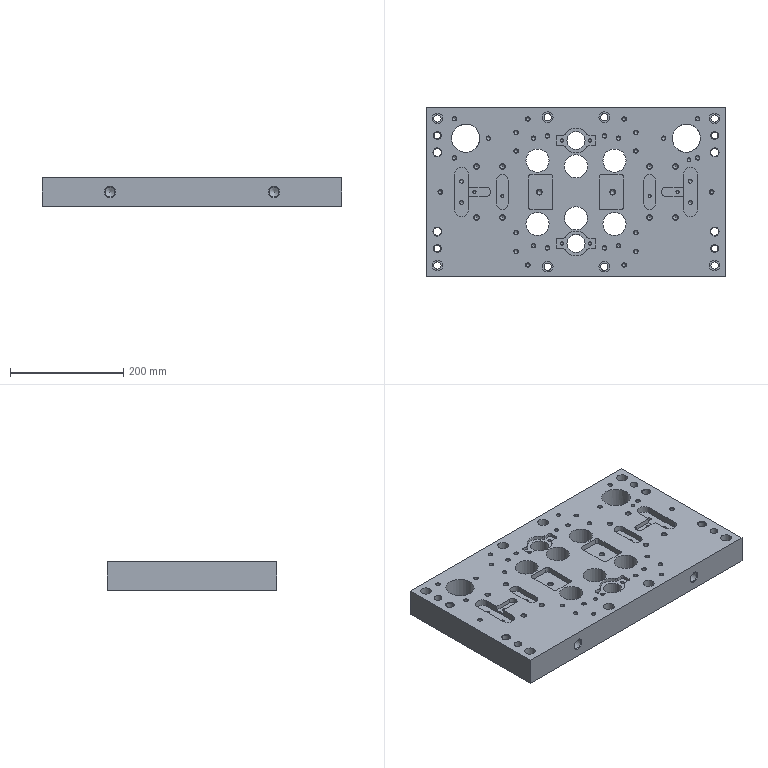Part | STEP file | gslz 2016.10.28-6_id14_x_t | 1 solid | 298 faces | box 530 x 300 x 50 mm | volume 6912423 mm3 | cylinder 131 | cone 107 | plane 60 | commonest cylinder face diameters 6.8 x29 8.5 x10 5 x8 6 x8 8 x8 10 x8